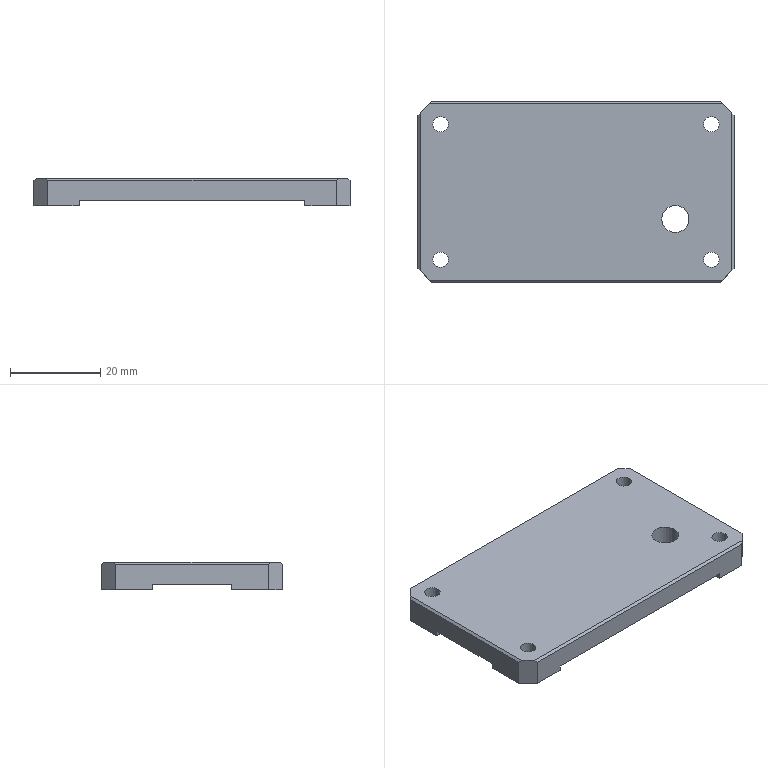Part | STEP file | 11-FG-Z01311 | 1 solid | 72 faces | box 70 x 40 x 6.2 mm | volume 13688 mm3 | plane 46 | cylinder 22 | cone 4 | commonest cylinder face diameters 3.4 x8 6.5 x8 2 x4 6 x2